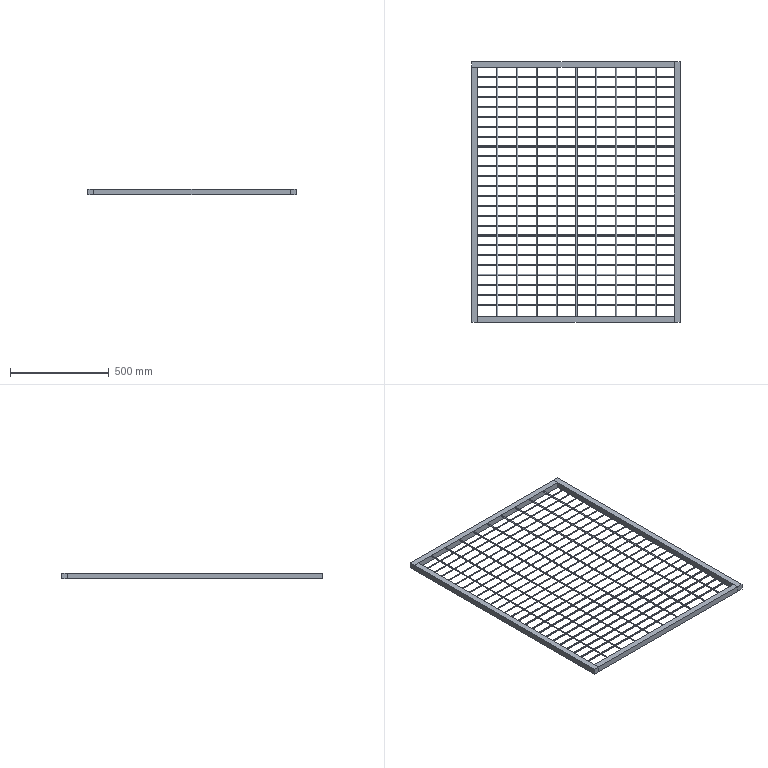Part | STEP file | 37 solids | 156 faces | box 1055 x 1320 x 30 mm | volume 5003767 mm3 | plane 90 | cylinder 66 | commonest cylinder face diameters 5.5 x66